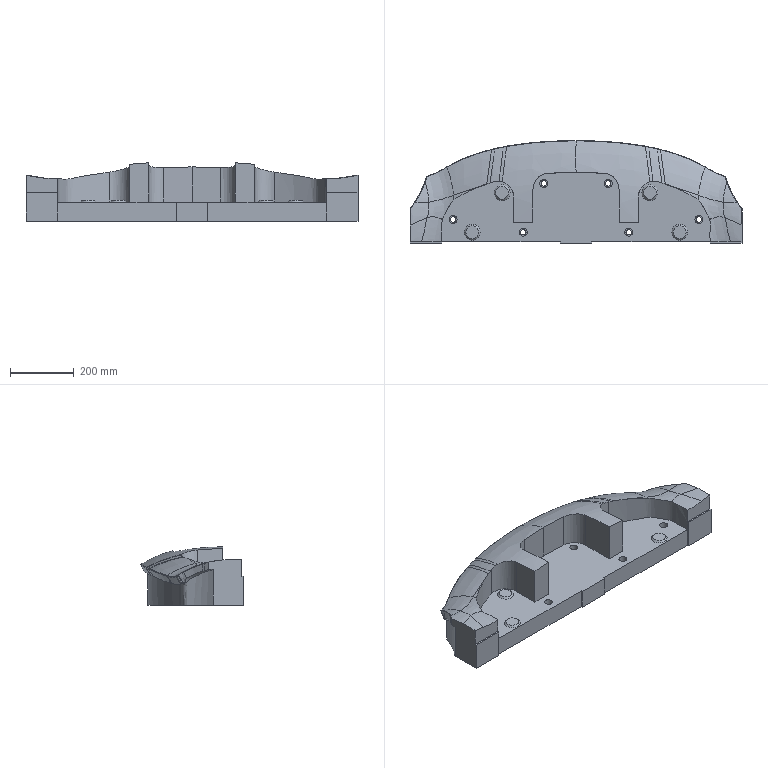Part | NX | features solid 2 | 1 solid | 209 faces | box 1040 x 322.115 x 183.006 mm | volume 23304178 mm3 | spline 124 | plane 51 | cylinder 30 | cone 4 | commonest cylinder face diameters 77 x8 17 x6 25 x6 40 x6 100 x4